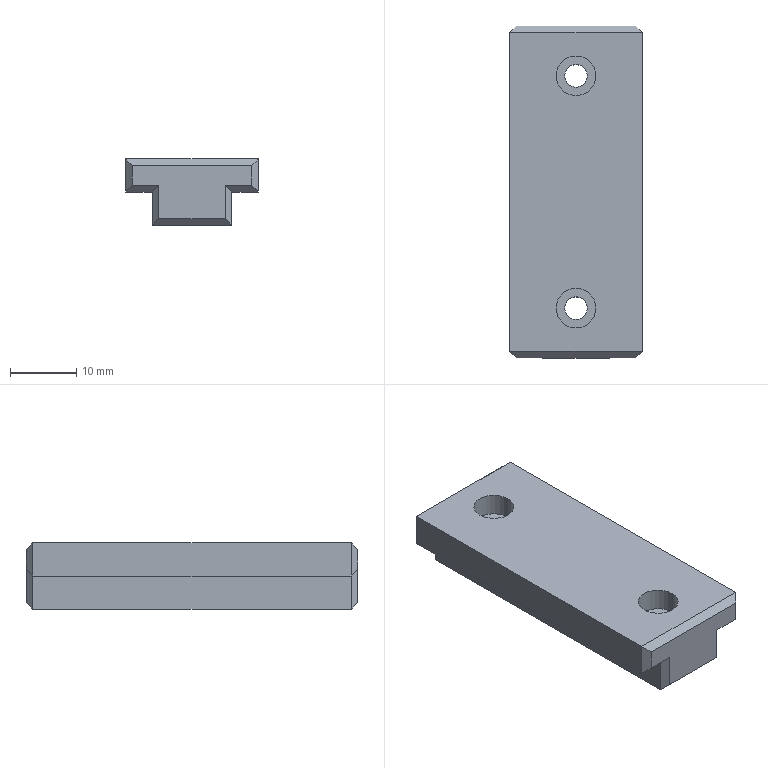Part | SolidWorks | features Chamfer 1, Extrusion 1, HoleWzd 1 | 1 solid | 36 faces | box 20 x 50 x 10 mm | volume 7631 mm3 | plane 28 | cylinder 8 | commonest cylinder face diameters 3.4 x4 6 x4
STEP:
#1=CARTESIAN_POINT('',(-3.,42.5,-3.4));
#2=VERTEX_POINT('',#1);
#3=CARTESIAN_POINT('',(3.,42.5,-3.4));
#4=VERTEX_POINT('',#3);
#5=CARTESIAN_POINT('',(0.,42.5,-3.4));
#6=DIRECTION('',(0.,0.,1.));
#7=DIRECTION('',(1.,0.,0.));
#8=AXIS2_PLACEMENT_3D('',#5,#6,#7);
#9=CIRCLE('',#8,3.);
#10=EDGE_CURVE('',#2,#4,#9,.T.);
#11=ORIENTED_EDGE('',*,*,#10,.F.);
#12=CARTESIAN_POINT('',(-3.,42.5,0.));
#13=VERTEX_POINT('',#12);
#14=CARTESIAN_POINT('',(-3.,42.5,0.));
#15=DIRECTION('',(0.,0.,1.));
#16=VECTOR('',#15,1000.);
#17=LINE('',#14,#16);
#18=EDGE_CURVE('',#2,#13,#17,.T.);
#19=ORIENTED_EDGE('',*,*,#18,.T.);
#20=CARTESIAN_POINT('',(3.,42.5,0.));
#21=VERTEX_POINT('',#20);
#22=CARTESIAN_POINT('',(0.,42.5,0.));
#23=DIRECTION('',(0.,0.,1.));
#24=DIRECTION('',(1.,0.,0.));
#25=AXIS2_PLACEMENT_3D('',#22,#23,#24);
#26=CIRCLE('',#25,3.);
#27=EDGE_CURVE('',#13,#21,#26,.T.);
#28=ORIENTED_EDGE('',*,*,#27,.T.);
#29=CARTESIAN_POINT('',(3.,42.5,0.));
#30=DIRECTION('',(0.,0.,1.));
#31=VECTOR('',#30,1000.);
#32=LINE('',#29,#31);
#33=EDGE_CURVE('',#4,#21,#32,.T.);
#34=ORIENTED_EDGE('',*,*,#33,.F.);
#35=EDGE_LOOP('',(#11,#19,#28,#34));
#36=FACE_OUTER_BOUND('',#35,.T.);
#37=CARTESIAN_POINT('',(0.,42.5,0.));
#38=DIRECTION('',(0.,0.,1.));
#39=DIRECTION('',(1.,0.,0.));
#40=AXIS2_PLACEMENT_3D('',#37,#38,#39);
#41=CYLINDRICAL_SURFACE('',#40,3.);
#42=ADVANCED_FACE('',(#36),#41,.F.);
#43=CARTESIAN_POINT('',(-1.7,42.5,-10.));
#44=VERTEX_POINT('',#43);
#45=CARTESIAN_POINT('',(1.7,42.5,-10.));
#46=VERTEX_POINT('',#45);
#47=CARTESIAN_POINT('',(0.,42.5,-10.));
#48=DIRECTION('',(0.,0.,1.));
#49=DIRECTION('',(1.,0.,0.));
#50=AXIS2_PLACEMENT_3D('',#47,#48,#49);
#51=CIRCLE('',#50,1.7);
#52=EDGE_CURVE('',#44,#46,#51,.T.);
#53=ORIENTED_EDGE('',*,*,#52,.F.);
#54=CARTESIAN_POINT('',(-1.7,42.5,-3.4));
#55=VERTEX_POINT('',#54);
#56=CARTESIAN_POINT('',(-1.7,42.5,0.));
#57=DIRECTION('',(0.,0.,1.));
#58=VECTOR('',#57,1000.);
#59=LINE('',#56,#58);
#60=EDGE_CURVE('',#44,#55,#59,.T.);
#61=ORIENTED_EDGE('',*,*,#60,.T.);
#62=CARTESIAN_POINT('',(1.7,42.5,-3.4));
#63=VERTEX_POINT('',#62);
#64=CARTESIAN_POINT('',(0.,42.5,-3.4));
#65=DIRECTION('',(0.,0.,1.));
#66=DIRECTION('',(1.,0.,0.));
#67=AXIS2_PLACEMENT_3D('',#64,#65,#66);
#68=CIRCLE('',#67,1.7);
#69=EDGE_CURVE('',#55,#63,#68,.T.);
#70=ORIENTED_EDGE('',*,*,#69,.T.);
#71=CARTESIAN_POINT('',(1.7,42.5,0.));
#72=DIRECTION('',(0.,0.,1.));
#73=VECTOR('',#72,1000.);
#74=LINE('',#71,#73);
#75=EDGE_CURVE('',#46,#63,#74,.T.);
#76=ORIENTED_EDGE('',*,*,#75,.F.);
#77=EDGE_LOOP('',(#53,#61,#70,#76));
#78=FACE_OUTER_BOUND('',#77,.T.);
#79=CARTESIAN_POINT('',(0.,42.5,0.));
#80=DIRECTION('',(0.,0.,1.));
#81=DIRECTION('',(1.,0.,0.));
#82=AXIS2_PLACEMENT_3D('',#79,#80,#81);
#83=CYLINDRICAL_SURFACE('',#82,1.7);
#84=ADVANCED_FACE('',(#78),#83,.F.);
#85=CARTESIAN_POINT('',(-3.,7.5,-3.4));
#86=VERTEX_POINT('',#85);
#87=CARTESIAN_POINT('',(3.,7.5,-3.4));
#88=VERTEX_POINT('',#87);
#89=CARTESIAN_POINT('',(0.,7.5,-3.4));
#90=DIRECTION('',(0.,0.,1.));
#91=DIRECTION('',(1.,0.,0.));
#92=AXIS2_PLACEMENT_3D('',#89,#90,#91);
#93=CIRCLE('',#92,3.);
#94=EDGE_CURVE('',#86,#88,#93,.T.);
#95=ORIENTED_EDGE('',*,*,#94,.F.);
#96=CARTESIAN_POINT('',(-3.,7.5,0.));
#97=VERTEX_POINT('',#96);
#98=CARTESIAN_POINT('',(-3.,7.5,0.));
#99=DIRECTION('',(0.,0.,1.));
#100=VECTOR('',#99,1000.);
#101=LINE('',#98,#100);
#102=EDGE_CURVE('',#86,#97,#101,.T.);
#103=ORIENTED_EDGE('',*,*,#102,.T.);
#104=CARTESIAN_POINT('',(3.,7.5,0.));
#105=VERTEX_POINT('',#104);
#106=CARTESIAN_POINT('',(0.,7.5,0.));
#107=DIRECTION('',(0.,0.,1.));
#108=DIRECTION('',(1.,0.,0.));
#109=AXIS2_PLACEMENT_3D('',#106,#107,#108);
#110=CIRCLE('',#109,3.);
#111=EDGE_CURVE('',#97,#105,#110,.T.);
#112=ORIENTED_EDGE('',*,*,#111,.T.);
#113=CARTESIAN_POINT('',(3.,7.5,0.));
#114=DIRECTION('',(0.,0.,1.));
#115=VECTOR('',#114,1000.);
#116=LINE('',#113,#115);
#117=EDGE_CURVE('',#88,#105,#116,.T.);
#118=ORIENTED_EDGE('',*,*,#117,.F.);
#119=EDGE_LOOP('',(#95,#103,#112,#118));
#120=FACE_OUTER_BOUND('',#119,.T.);
#121=CARTESIAN_POINT('',(0.,7.5,0.));
#122=DIRECTION('',(0.,0.,1.));
#123=DIRECTION('',(1.,0.,0.));
#124=AXIS2_PLACEMENT_3D('',#121,#122,#123);
#125=CYLINDRICAL_SURFACE('',#124,3.);
#126=ADVANCED_FACE('',(#120),#125,.F.);
#127=CARTESIAN_POINT('',(-1.7,7.5,-10.));
#128=VERTEX_POINT('',#127);
#129=CARTESIAN_POINT('',(1.7,7.5,-10.));
#130=VERTEX_POINT('',#129);
#131=CARTESIAN_POINT('',(0.,7.5,-10.));
#132=DIRECTION('',(0.,0.,1.));
#133=DIRECTION('',(1.,0.,0.));
#134=AXIS2_PLACEMENT_3D('',#131,#132,#133);
#135=CIRCLE('',#134,1.7);
#136=EDGE_CURVE('',#128,#130,#135,.T.);
#137=ORIENTED_EDGE('',*,*,#136,.F.);
#138=CARTESIAN_POINT('',(-1.7,7.5,-3.4));
#139=VERTEX_POINT('',#138);
#140=CARTESIAN_POINT('',(-1.7,7.5,0.));
#141=DIRECTION('',(0.,0.,1.));
#142=VECTOR('',#141,1000.);
#143=LINE('',#140,#142);
#144=EDGE_CURVE('',#128,#139,#143,.T.);
#145=ORIENTED_EDGE('',*,*,#144,.T.);
#146=CARTESIAN_POINT('',(1.7,7.5,-3.4));
#147=VERTEX_POINT('',#146);
#148=CARTESIAN_POINT('',(0.,7.5,-3.4));
#149=DIRECTION('',(0.,0.,1.));
#150=DIRECTION('',(1.,0.,0.));
#151=AXIS2_PLACEMENT_3D('',#148,#149,#150);
#152=CIRCLE('',#151,1.7);
#153=EDGE_CURVE('',#139,#147,#152,.T.);
#154=ORIENTED_EDGE('',*,*,#153,.T.);
#155=CARTESIAN_POINT('',(1.7,7.5,0.));
#156=DIRECTION('',(0.,0.,1.));
#157=VECTOR('',#156,1000.);
#158=LINE('',#155,#157);
#159=EDGE_CURVE('',#130,#147,#158,.T.);
#160=ORIENTED_EDGE('',*,*,#159,.F.);
#161=EDGE_LOOP('',(#137,#145,#154,#160));
#162=FACE_OUTER_BOUND('',#161,.T.);
#163=CARTESIAN_POINT('',(0.,7.5,0.));
#164=DIRECTION('',(0.,0.,1.));
#165=DIRECTION('',(1.,0.,0.));
#166=AXIS2_PLACEMENT_3D('',#163,#164,#165);
#167=CYLINDRICAL_SURFACE('',#166,1.7);
#168=ADVANCED_FACE('',(#162),#167,.F.);
#169=CARTESIAN_POINT('',(0.,7.5,0.));
#170=DIRECTION('',(0.,0.,1.));
#171=DIRECTION('',(1.,0.,0.));
#172=AXIS2_PLACEMENT_3D('',#169,#170,#171);
#173=CIRCLE('',#172,3.);
#174=EDGE_CURVE('',#105,#97,#173,.T.);
#175=ORIENTED_EDGE('',*,*,#174,.F.);
#176=ORIENTED_EDGE('',*,*,#111,.F.);
#177=EDGE_LOOP('',(#175,#176));
#178=FACE_BOUND('',#177,.T.);
#179=CARTESIAN_POINT('',(10.,49.,0.));
#180=VERTEX_POINT('',#179);
#181=CARTESIAN_POINT('',(10.,1.,0.));
#182=VERTEX_POINT('',#181);
#183=CARTESIAN_POINT('',(10.,50.,0.));
#184=DIRECTION('',(0.,-1.,0.));
#185=VECTOR('',#184,1000.);
#186=LINE('',#183,#185);
#187=EDGE_CURVE('',#180,#182,#186,.T.);
#188=ORIENTED_EDGE('',*,*,#187,.F.);
#189=CARTESIAN_POINT('',(-10.,49.,0.));
#190=VERTEX_POINT('',#189);
#191=CARTESIAN_POINT('',(10.,49.,0.));
#192=DIRECTION('',(-1.,0.,0.));
#193=VECTOR('',#192,1000.);
#194=LINE('',#191,#193);
#195=EDGE_CURVE('',#180,#190,#194,.T.);
#196=ORIENTED_EDGE('',*,*,#195,.T.);
#197=CARTESIAN_POINT('',(-10.,1.,0.));
#198=VERTEX_POINT('',#197);
#199=CARTESIAN_POINT('',(-10.,50.,0.));
#200=DIRECTION('',(0.,-1.,0.));
#201=VECTOR('',#200,1000.);
#202=LINE('',#199,#201);
#203=EDGE_CURVE('',#190,#198,#202,.T.);
#204=ORIENTED_EDGE('',*,*,#203,.T.);
#205=CARTESIAN_POINT('',(10.,1.,0.));
#206=DIRECTION('',(1.,0.,0.));
#207=VECTOR('',#206,1000.);
#208=LINE('',#205,#207);
#209=EDGE_CURVE('',#198,#182,#208,.T.);
#210=ORIENTED_EDGE('',*,*,#209,.T.);
#211=EDGE_LOOP('',(#188,#196,#204,#210));
#212=FACE_OUTER_BOUND('',#211,.T.);
#213=CARTESIAN_POINT('',(0.,42.5,0.));
#214=DIRECTION('',(0.,0.,1.));
#215=DIRECTION('',(1.,0.,0.));
#216=AXIS2_PLACEMENT_3D('',#213,#214,#215);
#217=CIRCLE('',#216,3.);
#218=EDGE_CURVE('',#21,#13,#217,.T.);
#219=ORIENTED_EDGE('',*,*,#218,.F.);
#220=ORIENTED_EDGE('',*,*,#27,.F.);
#221=EDGE_LOOP('',(#219,#220));
#222=FACE_BOUND('',#221,.T.);
#223=CARTESIAN_POINT('',(10.,50.,0.));
#224=DIRECTION('',(0.,0.,-1.));
#225=DIRECTION('',(-1.,0.,0.));
#226=AXIS2_PLACEMENT_3D('',#223,#224,#225);
#227=PLANE('',#226);
#228=ADVANCED_FACE('',(#178,#212,#222),#227,.F.);
#229=ORIENTED_EDGE('',*,*,#203,.F.);
#230=CARTESIAN_POINT('',(-10.,49.,-5.));
#231=VERTEX_POINT('',#230);
#232=CARTESIAN_POINT('',(-10.,49.,0.));
#233=DIRECTION('',(0.,0.,-1.));
#234=VECTOR('',#233,1000.);
#235=LINE('',#232,#234);
#236=EDGE_CURVE('',#190,#231,#235,.T.);
#237=ORIENTED_EDGE('',*,*,#236,.T.);
#238=CARTESIAN_POINT('',(-10.,1.,-5.));
#239=VERTEX_POINT('',#238);
#240=CARTESIAN_POINT('',(-10.,50.,-5.));
#241=DIRECTION('',(0.,-1.,0.));
#242=VECTOR('',#241,1000.);
#243=LINE('',#240,#242);
#244=EDGE_CURVE('',#231,#239,#243,.T.);
#245=ORIENTED_EDGE('',*,*,#244,.T.);
#246=CARTESIAN_POINT('',(-10.,1.,0.));
#247=DIRECTION('',(0.,0.,1.));
#248=VECTOR('',#247,1000.);
#249=LINE('',#246,#248);
#250=EDGE_CURVE('',#239,#198,#249,.T.);
#251=ORIENTED_EDGE('',*,*,#250,.T.);
#252=EDGE_LOOP('',(#229,#237,#245,#251));
#253=FACE_OUTER_BOUND('',#252,.T.);
#254=CARTESIAN_POINT('',(-10.,50.,0.));
#255=DIRECTION('',(1.,0.,0.));
#256=DIRECTION('',(0.,0.,-1.));
#257=AXIS2_PLACEMENT_3D('',#254,#255,#256);
#258=PLANE('',#257);
#259=ADVANCED_FACE('',(#253),#258,.F.);
#260=CARTESIAN_POINT('',(10.,49.,-5.));
#261=VERTEX_POINT('',#260);
#262=CARTESIAN_POINT('',(10.,1.,-5.));
#263=VERTEX_POINT('',#262);
#264=CARTESIAN_POINT('',(10.,50.,-5.));
#265=DIRECTION('',(0.,-1.,0.));
#266=VECTOR('',#265,1000.);
#267=LINE('',#264,#266);
#268=EDGE_CURVE('',#261,#263,#267,.T.);
#269=ORIENTED_EDGE('',*,*,#268,.F.);
#270=CARTESIAN_POINT('',(10.,49.,0.));
#271=DIRECTION('',(0.,0.,1.));
#272=VECTOR('',#271,1000.);
#273=LINE('',#270,#272);
#274=EDGE_CURVE('',#261,#180,#273,.T.);
#275=ORIENTED_EDGE('',*,*,#274,.T.);
#276=ORIENTED_EDGE('',*,*,#187,.T.);
#277=CARTESIAN_POINT('',(10.,1.,-5.));
#278=DIRECTION('',(0.,0.,-1.));
#279=VECTOR('',#278,1000.);
#280=LINE('',#277,#279);
#281=EDGE_CURVE('',#182,#263,#280,.T.);
#282=ORIENTED_EDGE('',*,*,#281,.T.);
#283=EDGE_LOOP('',(#269,#275,#276,#282));
#284=FACE_OUTER_BOUND('',#283,.T.);
#285=CARTESIAN_POINT('',(10.,50.,0.));
#286=DIRECTION('',(-1.,0.,0.));
#287=DIRECTION('',(0.,0.,1.));
#288=AXIS2_PLACEMENT_3D('',#285,#286,#287);
#289=PLANE('',#288);
#290=ADVANCED_FACE('',(#284),#289,.F.);
#291=CARTESIAN_POINT('',(6.,49.,-5.));
#292=VERTEX_POINT('',#291);
#293=CARTESIAN_POINT('',(6.,1.,-5.));
#294=VERTEX_POINT('',#293);
#295=CARTESIAN_POINT('',(6.,50.,-5.));
#296=DIRECTION('',(0.,-1.,0.));
#297=VECTOR('',#296,1000.);
#298=LINE('',#295,#297);
#299=EDGE_CURVE('',#292,#294,#298,.T.);
#300=ORIENTED_EDGE('',*,*,#299,.F.);
#301=CARTESIAN_POINT('',(10.,49.,-5.));
#302=DIRECTION('',(1.,0.,0.));
#303=VECTOR('',#302,1000.);
#304=LINE('',#301,#303);
#305=EDGE_CURVE('',#292,#261,#304,.T.);
#306=ORIENTED_EDGE('',*,*,#305,.T.);
#307=ORIENTED_EDGE('',*,*,#268,.T.);
#308=CARTESIAN_POINT('',(6.,1.,-5.));
#309=DIRECTION('',(-1.,0.,0.));
#310=VECTOR('',#309,1000.);
#311=LINE('',#308,#310);
#312=EDGE_CURVE('',#263,#294,#311,.T.);
#313=ORIENTED_EDGE('',*,*,#312,.T.);
#314=EDGE_LOOP('',(#300,#306,#307,#313));
#315=FACE_OUTER_BOUND('',#314,.T.);
#316=CARTESIAN_POINT('',(10.,50.,-5.));
#317=DIRECTION('',(0.,0.,1.));
#318=DIRECTION('',(1.,0.,0.));
#319=AXIS2_PLACEMENT_3D('',#316,#317,#318);
#320=PLANE('',#319);
#321=ADVANCED_FACE('',(#315),#320,.F.);
#322=CARTESIAN_POINT('',(6.,49.,-10.));
#323=VERTEX_POINT('',#322);
#324=CARTESIAN_POINT('',(6.,1.,-10.));
#325=VERTEX_POINT('',#324);
#326=CARTESIAN_POINT('',(6.,50.,-10.));
#327=DIRECTION('',(0.,-1.,0.));
#328=VECTOR('',#327,1000.);
#329=LINE('',#326,#328);
#330=EDGE_CURVE('',#323,#325,#329,.T.);
#331=ORIENTED_EDGE('',*,*,#330,.F.);
#332=CARTESIAN_POINT('',(6.,49.,-5.));
#333=DIRECTION('',(0.,0.,1.));
#334=VECTOR('',#333,1000.);
#335=LINE('',#332,#334);
#336=EDGE_CURVE('',#323,#292,#335,.T.);
#337=ORIENTED_EDGE('',*,*,#336,.T.);
#338=ORIENTED_EDGE('',*,*,#299,.T.);
#339=CARTESIAN_POINT('',(6.,1.,-10.));
#340=DIRECTION('',(0.,0.,-1.));
#341=VECTOR('',#340,1000.);
#342=LINE('',#339,#341);
#343=EDGE_CURVE('',#294,#325,#342,.T.);
#344=ORIENTED_EDGE('',*,*,#343,.T.);
#345=EDGE_LOOP('',(#331,#337,#338,#344));
#346=FACE_OUTER_BOUND('',#345,.T.);
#347=CARTESIAN_POINT('',(6.,50.,-5.));
#348=DIRECTION('',(-1.,0.,0.));
#349=DIRECTION('',(0.,0.,1.));
#350=AXIS2_PLACEMENT_3D('',#347,#348,#349);
#351=PLANE('',#350);
#352=ADVANCED_FACE('',(#346),#351,.F.);
#353=CARTESIAN_POINT('',(0.,42.5,-10.));
#354=DIRECTION('',(0.,0.,1.));
#355=DIRECTION('',(1.,0.,0.));
#356=AXIS2_PLACEMENT_3D('',#353,#354,#355);
#357=CIRCLE('',#356,1.7);
#358=EDGE_CURVE('',#46,#44,#357,.T.);
#359=ORIENTED_EDGE('',*,*,#358,.T.);
#360=ORIENTED_EDGE('',*,*,#52,.T.);
#361=EDGE_LOOP('',(#359,#360));
#362=FACE_BOUND('',#361,.T.);
#363=CARTESIAN_POINT('',(0.,7.5,-10.));
#364=DIRECTION('',(0.,0.,1.));
#365=DIRECTION('',(1.,0.,0.));
#366=AXIS2_PLACEMENT_3D('',#363,#364,#365);
#367=CIRCLE('',#366,1.7);
#368=EDGE_CURVE('',#130,#128,#367,.T.);
#369=ORIENTED_EDGE('',*,*,#368,.T.);
#370=ORIENTED_EDGE('',*,*,#136,.T.);
#371=EDGE_LOOP('',(#369,#370));
#372=FACE_BOUND('',#371,.T.);
#373=CARTESIAN_POINT('',(-6.,49.,-10.));
#374=VERTEX_POINT('',#373);
#375=CARTESIAN_POINT('',(-6.,1.,-10.));
#376=VERTEX_POINT('',#375);
#377=CARTESIAN_POINT('',(-6.,50.,-10.));
#378=DIRECTION('',(0.,-1.,0.));
#379=VECTOR('',#378,1000.);
#380=LINE('',#377,#379);
#381=EDGE_CURVE('',#374,#376,#380,.T.);
#382=ORIENTED_EDGE('',*,*,#381,.F.);
#383=CARTESIAN_POINT('',(-6.,49.,-10.));
#384=DIRECTION('',(1.,0.,0.));
#385=VECTOR('',#384,1000.);
#386=LINE('',#383,#385);
#387=EDGE_CURVE('',#374,#323,#386,.T.);
#388=ORIENTED_EDGE('',*,*,#387,.T.);
#389=ORIENTED_EDGE('',*,*,#330,.T.);
#390=CARTESIAN_POINT('',(-6.,1.,-10.));
#391=DIRECTION('',(-1.,0.,0.));
#392=VECTOR('',#391,1000.);
#393=LINE('',#390,#392);
#394=EDGE_CURVE('',#325,#376,#393,.T.);
#395=ORIENTED_EDGE('',*,*,#394,.T.);
#396=EDGE_LOOP('',(#382,#388,#389,#395));
#397=FACE_OUTER_BOUND('',#396,.T.);
#398=CARTESIAN_POINT('',(-6.,50.,-10.));
#399=DIRECTION('',(0.,0.,1.));
#400=DIRECTION('',(1.,0.,0.));
#401=AXIS2_PLACEMENT_3D('',#398,#399,#400);
#402=PLANE('',#401);
#403=ADVANCED_FACE('',(#362,#372,#397),#402,.F.);
#404=CARTESIAN_POINT('',(-6.,49.,-5.));
#405=VERTEX_POINT('',#404);
#406=CARTESIAN_POINT('',(-6.,1.,-5.));
#407=VERTEX_POINT('',#406);
#408=CARTESIAN_POINT('',(-6.,50.,-5.));
#409=DIRECTION('',(0.,-1.,0.));
#410=VECTOR('',#409,1000.);
#411=LINE('',#408,#410);
#412=EDGE_CURVE('',#405,#407,#411,.T.);
#413=ORIENTED_EDGE('',*,*,#412,.F.);
#414=CARTESIAN_POINT('',(-6.,49.,-5.));
#415=DIRECTION('',(0.,0.,-1.));
#416=VECTOR('',#415,1000.);
#417=LINE('',#414,#416);
#418=EDGE_CURVE('',#405,#374,#417,.T.);
#419=ORIENTED_EDGE('',*,*,#418,.T.);
#420=ORIENTED_EDGE('',*,*,#381,.T.);
#421=CARTESIAN_POINT('',(-6.,1.,-5.));
#422=DIRECTION('',(0.,0.,1.));
#423=VECTOR('',#422,1000.);
#424=LINE('',#421,#423);
#425=EDGE_CURVE('',#376,#407,#424,.T.);
#426=ORIENTED_EDGE('',*,*,#425,.T.);
#427=EDGE_LOOP('',(#413,#419,#420,#426));
#428=FACE_OUTER_BOUND('',#427,.T.);
#429=CARTESIAN_POINT('',(-6.,50.,-5.));
#430=DIRECTION('',(1.,0.,0.));
#431=DIRECTION('',(0.,0.,-1.));
#432=AXIS2_PLACEMENT_3D('',#429,#430,#431);
#433=PLANE('',#432);
#434=ADVANCED_FACE('',(#428),#433,.F.);
#435=ORIENTED_EDGE('',*,*,#244,.F.);
#436=CARTESIAN_POINT('',(-10.,49.,-5.));
#437=DIRECTION('',(1.,0.,0.));
#438=VECTOR('',#437,1000.);
#439=LINE('',#436,#438);
#440=EDGE_CURVE('',#231,#405,#439,.T.);
#441=ORIENTED_EDGE('',*,*,#440,.T.);
#442=ORIENTED_EDGE('',*,*,#412,.T.);
#443=CARTESIAN_POINT('',(-10.,1.,-5.));
#444=DIRECTION('',(-1.,0.,0.));
#445=VECTOR('',#444,1000.);
#446=LINE('',#443,#445);
#447=EDGE_CURVE('',#407,#239,#446,.T.);
#448=ORIENTED_EDGE('',*,*,#447,.T.);
#449=EDGE_LOOP('',(#435,#441,#442,#448));
#450=FACE_OUTER_BOUND('',#449,.T.);
#451=CARTESIAN_POINT('',(-10.,50.,-5.));
#452=DIRECTION('',(0.,0.,1.));
#453=DIRECTION('',(1.,0.,0.));
#454=AXIS2_PLACEMENT_3D('',#451,#452,#453);
#455=PLANE('',#454);
#456=ADVANCED_FACE('',(#450),#455,.F.);
#457=CARTESIAN_POINT('',(-9.,50.,-4.));
#458=VERTEX_POINT('',#457);
#459=CARTESIAN_POINT('',(-9.,50.,-1.));
#460=VERTEX_POINT('',#459);
#461=CARTESIAN_POINT('',(-9.,50.,0.));
#462=DIRECTION('',(0.,0.,1.));
#463=VECTOR('',#462,1000.);
#464=LINE('',#461,#463);
#465=EDGE_CURVE('',#458,#460,#464,.T.);
#466=ORIENTED_EDGE('',*,*,#465,.T.);
#467=CARTESIAN_POINT('',(9.,50.,-1.));
#468=VERTEX_POINT('',#467);
#469=CARTESIAN_POINT('',(0.,50.,-1.));
#470=DIRECTION('',(1.,0.,0.));
#471=VECTOR('',#470,1000.);
#472=LINE('',#469,#471);
#473=EDGE_CURVE('',#460,#468,#472,.T.);
#474=ORIENTED_EDGE('',*,*,#473,.T.);
#475=CARTESIAN_POINT('',(9.,50.,-4.));
#476=VERTEX_POINT('',#475);
#477=CARTESIAN_POINT('',(9.,50.,0.));
#478=DIRECTION('',(0.,0.,-1.));
#479=VECTOR('',#478,1000.);
#480=LINE('',#477,#479);
#481=EDGE_CURVE('',#468,#476,#480,.T.);
#482=ORIENTED_EDGE('',*,*,#481,.T.);
#483=CARTESIAN_POINT('',(5.,50.,-4.));
#484=VERTEX_POINT('',#483);
#485=CARTESIAN_POINT('',(0.,50.,-4.));
#486=DIRECTION('',(-1.,0.,0.));
#487=VECTOR('',#486,1000.);
#488=LINE('',#485,#487);
#489=EDGE_CURVE('',#476,#484,#488,.T.);
#490=ORIENTED_EDGE('',*,*,#489,.T.);
#491=CARTESIAN_POINT('',(5.,50.,-9.));
#492=VERTEX_POINT('',#491);
#493=CARTESIAN_POINT('',(5.,50.,0.));
#494=DIRECTION('',(0.,0.,-1.));
#495=VECTOR('',#494,1000.);
#496=LINE('',#493,#495);
#497=EDGE_CURVE('',#484,#492,#496,.T.);
#498=ORIENTED_EDGE('',*,*,#497,.T.);
#499=CARTESIAN_POINT('',(-5.,50.,-9.));
#500=VERTEX_POINT('',#499);
#501=CARTESIAN_POINT('',(0.,50.,-9.));
#502=DIRECTION('',(-1.,0.,0.));
#503=VECTOR('',#502,1000.);
#504=LINE('',#501,#503);
#505=EDGE_CURVE('',#492,#500,#504,.T.);
#506=ORIENTED_EDGE('',*,*,#505,.T.);
#507=CARTESIAN_POINT('',(-5.,50.,-4.));
#508=VERTEX_POINT('',#507);
#509=CARTESIAN_POINT('',(-5.,50.,0.));
#510=DIRECTION('',(0.,0.,1.));
#511=VECTOR('',#510,1000.);
#512=LINE('',#509,#511);
#513=EDGE_CURVE('',#500,#508,#512,.T.);
#514=ORIENTED_EDGE('',*,*,#513,.T.);
#515=CARTESIAN_POINT('',(0.,50.,-4.));
#516=DIRECTION('',(-1.,0.,0.));
#517=VECTOR('',#516,1000.);
#518=LINE('',#515,#517);
#519=EDGE_CURVE('',#508,#458,#518,.T.);
#520=ORIENTED_EDGE('',*,*,#519,.T.);
#521=EDGE_LOOP('',(#466,#474,#482,#490,#498,#506,#514,#520));
#522=FACE_OUTER_BOUND('',#521,.T.);
#523=CARTESIAN_POINT('',(0.,50.,0.));
#524=DIRECTION('',(0.,-1.,0.));
#525=DIRECTION('',(0.,0.,-1.));
#526=AXIS2_PLACEMENT_3D('',#523,#524,#525);
#527=PLANE('',#526);
#528=ADVANCED_FACE('',(#522),#527,.F.);
#529=CARTESIAN_POINT('',(9.,0.,-4.));
#530=VERTEX_POINT('',#529);
#531=CARTESIAN_POINT('',(9.,0.,-1.));
#532=VERTEX_POINT('',#531);
#533=CARTESIAN_POINT('',(9.,0.,0.));
#534=DIRECTION('',(0.,0.,1.));
#535=VECTOR('',#534,1000.);
#536=LINE('',#533,#535);
#537=EDGE_CURVE('',#530,#532,#536,.T.);
#538=ORIENTED_EDGE('',*,*,#537,.T.);
#539=CARTESIAN_POINT('',(-9.,0.,-1.));
#540=VERTEX_POINT('',#539);
#541=CARTESIAN_POINT('',(-10.,0.,-1.));
#542=DIRECTION('',(-1.,0.,0.));
#543=VECTOR('',#542,1000.);
#544=LINE('',#541,#543);
#545=EDGE_CURVE('',#532,#540,#544,.T.);
#546=ORIENTED_EDGE('',*,*,#545,.T.);
#547=CARTESIAN_POINT('',(-9.,0.,-4.));
#548=VERTEX_POINT('',#547);
#549=CARTESIAN_POINT('',(-9.,0.,-5.));
#550=DIRECTION('',(0.,0.,-1.));
#551=VECTOR('',#550,1000.);
#552=LINE('',#549,#551);
#553=EDGE_CURVE('',#540,#548,#552,.T.);
#554=ORIENTED_EDGE('',*,*,#553,.T.);
#555=CARTESIAN_POINT('',(-5.,0.,-4.));
#556=VERTEX_POINT('',#555);
#557=CARTESIAN_POINT('',(-6.,0.,-4.));
#558=DIRECTION('',(1.,0.,0.));
#559=VECTOR('',#558,1000.);
#560=LINE('',#557,#559);
#561=EDGE_CURVE('',#548,#556,#560,.T.);
#562=ORIENTED_EDGE('',*,*,#561,.T.);
#563=CARTESIAN_POINT('',(-5.,0.,-9.));
#564=VERTEX_POINT('',#563);
#565=CARTESIAN_POINT('',(-5.,0.,-10.));
#566=DIRECTION('',(0.,0.,-1.));
#567=VECTOR('',#566,1000.);
#568=LINE('',#565,#567);
#569=EDGE_CURVE('',#556,#564,#568,.T.);
#570=ORIENTED_EDGE('',*,*,#569,.T.);
#571=CARTESIAN_POINT('',(5.,0.,-9.));
#572=VERTEX_POINT('',#571);
#573=CARTESIAN_POINT('',(6.,0.,-9.));
#574=DIRECTION('',(1.,0.,0.));
#575=VECTOR('',#574,1000.);
#576=LINE('',#573,#575);
#577=EDGE_CURVE('',#564,#572,#576,.T.);
#578=ORIENTED_EDGE('',*,*,#577,.T.);
#579=CARTESIAN_POINT('',(5.,0.,-4.));
#580=VERTEX_POINT('',#579);
#581=CARTESIAN_POINT('',(5.,0.,-5.));
#582=DIRECTION('',(0.,0.,1.));
#583=VECTOR('',#582,1000.);
#584=LINE('',#581,#583);
#585=EDGE_CURVE('',#572,#580,#584,.T.);
#586=ORIENTED_EDGE('',*,*,#585,.T.);
#587=CARTESIAN_POINT('',(10.,0.,-4.));
#588=DIRECTION('',(1.,0.,0.));
#589=VECTOR('',#588,1000.);
#590=LINE('',#587,#589);
#591=EDGE_CURVE('',#580,#530,#590,.T.);
#592=ORIENTED_EDGE('',*,*,#591,.T.);
#593=EDGE_LOOP('',(#538,#546,#554,#562,#570,#578,#586,#592));
#594=FACE_OUTER_BOUND('',#593,.T.);
#595=CARTESIAN_POINT('',(0.,0.,0.));
#596=DIRECTION('',(0.,-1.,0.));
#597=DIRECTION('',(0.,0.,-1.));
#598=AXIS2_PLACEMENT_3D('',#595,#596,#597);
#599=PLANE('',#598);
#600=ADVANCED_FACE('',(#594),#599,.T.);
#601=CARTESIAN_POINT('',(2.,53.,-6.));
#602=DIRECTION('',(-0.5774,0.5774,0.5774));
#603=VECTOR('',#602,1000.);
#604=LINE('',#601,#603);
#605=EDGE_CURVE('',#323,#492,#604,.T.);
#606=ORIENTED_EDGE('',*,*,#605,.F.);
#607=ORIENTED_EDGE('',*,*,#387,.F.);
#608=CARTESIAN_POINT('',(-3.333,51.667,-7.333));
#609=DIRECTION('',(-0.5774,-0.5774,-0.5774));
#610=VECTOR('',#609,1000.);
#611=LINE('',#608,#610);
#612=EDGE_CURVE('',#500,#374,#611,.T.);
#613=ORIENTED_EDGE('',*,*,#612,.F.);
#614=ORIENTED_EDGE('',*,*,#505,.F.);
#615=EDGE_LOOP('',(#606,#607,#613,#614));
#616=FACE_OUTER_BOUND('',#615,.T.);
#617=CARTESIAN_POINT('',(0.,50.,-9.));
#618=DIRECTION('',(0.,-0.7071,0.7071));
#619=DIRECTION('',(-1.,0.,0.));
#620=AXIS2_PLACEMENT_3D('',#617,#618,#619);
#621=PLANE('',#620);
#622=ADVANCED_FACE('',(#616),#621,.F.);
#623=ORIENTED_EDGE('',*,*,#612,.T.);
#624=ORIENTED_EDGE('',*,*,#418,.F.);
#625=CARTESIAN_POINT('',(-3.333,51.667,-2.333));
#626=DIRECTION('',(-0.5774,-0.5774,-0.5774));
#627=VECTOR('',#626,1000.);
#628=LINE('',#625,#627);
#629=EDGE_CURVE('',#508,#405,#628,.T.);
#630=ORIENTED_EDGE('',*,*,#629,.F.);
#631=ORIENTED_EDGE('',*,*,#513,.F.);
#632=EDGE_LOOP('',(#623,#624,#630,#631));
#633=FACE_OUTER_BOUND('',#632,.T.);
#634=CARTESIAN_POINT('',(-5.,50.,0.));
#635=DIRECTION('',(0.7071,-0.7071,0.));
#636=DIRECTION('',(0.,0.,1.));
#637=AXIS2_PLACEMENT_3D('',#634,#635,#636);
#638=PLANE('',#637);
#639=ADVANCED_FACE('',(#633),#638,.F.);
#640=ORIENTED_EDGE('',*,*,#605,.T.);
#641=ORIENTED_EDGE('',*,*,#497,.F.);
#642=CARTESIAN_POINT('',(3.667,51.333,-2.667));
#643=DIRECTION('',(-0.5774,0.5774,0.5774));
#644=VECTOR('',#643,1000.);
#645=LINE('',#642,#644);
#646=EDGE_CURVE('',#292,#484,#645,.T.);
#647=ORIENTED_EDGE('',*,*,#646,.F.);
#648=ORIENTED_EDGE('',*,*,#336,.F.);
#649=EDGE_LOOP('',(#640,#641,#647,#648));
#650=FACE_OUTER_BOUND('',#649,.T.);
#651=CARTESIAN_POINT('',(5.,50.,0.));
#652=DIRECTION('',(-0.7071,-0.7071,0.));
#653=DIRECTION('',(0.,0.,-1.));
#654=AXIS2_PLACEMENT_3D('',#651,#652,#653);
#655=PLANE('',#654);
#656=ADVANCED_FACE('',(#650),#655,.F.);
#657=ORIENTED_EDGE('',*,*,#629,.T.);
#658=ORIENTED_EDGE('',*,*,#440,.F.);
#659=CARTESIAN_POINT('',(-6.,53.,-1.));
#660=DIRECTION('',(-0.5774,-0.5774,-0.5774));
#661=VECTOR('',#660,1000.);
#662=LINE('',#659,#661);
#663=EDGE_CURVE('',#458,#231,#662,.T.);
#664=ORIENTED_EDGE('',*,*,#663,.F.);
#665=ORIENTED_EDGE('',*,*,#519,.F.);
#666=EDGE_LOOP('',(#657,#658,#664,#665));
#667=FACE_OUTER_BOUND('',#666,.T.);
#668=CARTESIAN_POINT('',(0.,50.,-4.));
#669=DIRECTION('',(0.,-0.7071,0.7071));
#670=DIRECTION('',(-1.,0.,0.));
#671=AXIS2_PLACEMENT_3D('',#668,#669,#670);
#672=PLANE('',#671);
#673=ADVANCED_FACE('',(#667),#672,.F.);
#674=ORIENTED_EDGE('',*,*,#646,.T.);
#675=ORIENTED_EDGE('',*,*,#489,.F.);
#676=CARTESIAN_POINT('',(7.667,51.333,-2.667));
#677=DIRECTION('',(-0.5774,0.5774,0.5774));
#678=VECTOR('',#677,1000.);
#679=LINE('',#676,#678);
#680=EDGE_CURVE('',#261,#476,#679,.T.);
#681=ORIENTED_EDGE('',*,*,#680,.F.);
#682=ORIENTED_EDGE('',*,*,#305,.F.);
#683=EDGE_LOOP('',(#674,#675,#681,#682));
#684=FACE_OUTER_BOUND('',#683,.T.);
#685=CARTESIAN_POINT('',(0.,50.,-4.));
#686=DIRECTION('',(0.,-0.7071,0.7071));
#687=DIRECTION('',(-1.,0.,0.));
#688=AXIS2_PLACEMENT_3D('',#685,#686,#687);
#689=PLANE('',#688);
#690=ADVANCED_FACE('',(#684),#689,.F.);
#691=ORIENTED_EDGE('',*,*,#663,.T.);
#692=ORIENTED_EDGE('',*,*,#236,.F.);
#693=CARTESIAN_POINT('',(-9.333,49.667,-0.6667));
#694=DIRECTION('',(-0.5774,-0.5774,0.5774));
#695=VECTOR('',#694,1000.);
#696=LINE('',#693,#695);
#697=EDGE_CURVE('',#460,#190,#696,.T.);
#698=ORIENTED_EDGE('',*,*,#697,.F.);
#699=ORIENTED_EDGE('',*,*,#465,.F.);
#700=EDGE_LOOP('',(#691,#692,#698,#699));
#701=FACE_OUTER_BOUND('',#700,.T.);
#702=CARTESIAN_POINT('',(-9.,50.,0.));
#703=DIRECTION('',(0.7071,-0.7071,0.));
#704=DIRECTION('',(0.,0.,1.));
#705=AXIS2_PLACEMENT_3D('',#702,#703,#704);
#706=PLANE('',#705);
#707=ADVANCED_FACE('',(#701),#706,.F.);
#708=ORIENTED_EDGE('',*,*,#680,.T.);
#709=ORIENTED_EDGE('',*,*,#481,.F.);
#710=CARTESIAN_POINT('',(9.333,49.667,-0.6667));
#711=DIRECTION('',(-0.5774,0.5774,-0.5774));
#712=VECTOR('',#711,1000.);
#713=LINE('',#710,#712);
#714=EDGE_CURVE('',#180,#468,#713,.T.);
#715=ORIENTED_EDGE('',*,*,#714,.F.);
#716=ORIENTED_EDGE('',*,*,#274,.F.);
#717=EDGE_LOOP('',(#708,#709,#715,#716));
#718=FACE_OUTER_BOUND('',#717,.T.);
#719=CARTESIAN_POINT('',(9.,50.,0.));
#720=DIRECTION('',(-0.7071,-0.7071,0.));
#721=DIRECTION('',(0.,0.,-1.));
#722=AXIS2_PLACEMENT_3D('',#719,#720,#721);
#723=PLANE('',#722);
#724=ADVANCED_FACE('',(#718),#723,.F.);
#725=ORIENTED_EDGE('',*,*,#697,.T.);
#726=ORIENTED_EDGE('',*,*,#195,.F.);
#727=ORIENTED_EDGE('',*,*,#714,.T.);
#728=ORIENTED_EDGE('',*,*,#473,.F.);
#729=EDGE_LOOP('',(#725,#726,#727,#728));
#730=FACE_OUTER_BOUND('',#729,.T.);
#731=CARTESIAN_POINT('',(0.,50.,-1.));
#732=DIRECTION('',(0.,-0.7071,-0.7071));
#733=DIRECTION('',(1.,0.,0.));
#734=AXIS2_PLACEMENT_3D('',#731,#732,#733);
#735=PLANE('',#734);
#736=ADVANCED_FACE('',(#730),#735,.F.);
#737=CARTESIAN_POINT('',(2.,-3.,-6.));
#738=DIRECTION('',(0.5774,0.5774,-0.5774));
#739=VECTOR('',#738,1000.);
#740=LINE('',#737,#739);
#741=EDGE_CURVE('',#572,#325,#740,.T.);
#742=ORIENTED_EDGE('',*,*,#741,.F.);
#743=ORIENTED_EDGE('',*,*,#577,.F.);
#744=CARTESIAN_POINT('',(-6.,1.,-10.));
#745=DIRECTION('',(0.5774,-0.5774,0.5774));
#746=VECTOR('',#745,1000.);
#747=LINE('',#744,#746);
#748=EDGE_CURVE('',#376,#564,#747,.T.);
#749=ORIENTED_EDGE('',*,*,#748,.F.);
#750=ORIENTED_EDGE('',*,*,#394,.F.);
#751=EDGE_LOOP('',(#742,#743,#749,#750));
#752=FACE_OUTER_BOUND('',#751,.T.);
#753=CARTESIAN_POINT('',(-6.,1.,-10.));
#754=DIRECTION('',(0.,-0.7071,-0.7071));
#755=DIRECTION('',(1.,0.,0.));
#756=AXIS2_PLACEMENT_3D('',#753,#754,#755);
#757=PLANE('',#756);
#758=ADVANCED_FACE('',(#752),#757,.T.);
#759=ORIENTED_EDGE('',*,*,#748,.T.);
#760=ORIENTED_EDGE('',*,*,#569,.F.);
#761=CARTESIAN_POINT('',(-7.333,2.333,-6.333));
#762=DIRECTION('',(0.5774,-0.5774,0.5774));
#763=VECTOR('',#762,1000.);
#764=LINE('',#761,#763);
#765=EDGE_CURVE('',#407,#556,#764,.T.);
#766=ORIENTED_EDGE('',*,*,#765,.F.);
#767=ORIENTED_EDGE('',*,*,#425,.F.);
#768=EDGE_LOOP('',(#759,#760,#766,#767));
#769=FACE_OUTER_BOUND('',#768,.T.);
#770=CARTESIAN_POINT('',(-6.,1.,-5.));
#771=DIRECTION('',(-0.7071,-0.7071,0.));
#772=DIRECTION('',(0.,0.,-1.));
#773=AXIS2_PLACEMENT_3D('',#770,#771,#772);
#774=PLANE('',#773);
#775=ADVANCED_FACE('',(#769),#774,.T.);
#776=ORIENTED_EDGE('',*,*,#741,.T.);
#777=ORIENTED_EDGE('',*,*,#343,.F.);
#778=CARTESIAN_POINT('',(7.333,2.333,-6.333));
#779=DIRECTION('',(0.5774,0.5774,-0.5774));
#780=VECTOR('',#779,1000.);
#781=LINE('',#778,#780);
#782=EDGE_CURVE('',#580,#294,#781,.T.);
#783=ORIENTED_EDGE('',*,*,#782,.F.);
#784=ORIENTED_EDGE('',*,*,#585,.F.);
#785=EDGE_LOOP('',(#776,#777,#783,#784));
#786=FACE_OUTER_BOUND('',#785,.T.);
#787=CARTESIAN_POINT('',(6.,1.,-5.));
#788=DIRECTION('',(0.7071,-0.7071,0.));
#789=DIRECTION('',(0.,0.,1.));
#790=AXIS2_PLACEMENT_3D('',#787,#788,#789);
#791=PLANE('',#790);
#792=ADVANCED_FACE('',(#786),#791,.T.);
#793=ORIENTED_EDGE('',*,*,#765,.T.);
#794=ORIENTED_EDGE('',*,*,#561,.F.);
#795=CARTESIAN_POINT('',(-10.,1.,-5.));
#796=DIRECTION('',(0.5774,-0.5774,0.5774));
#797=VECTOR('',#796,1000.);
#798=LINE('',#795,#797);
#799=EDGE_CURVE('',#239,#548,#798,.T.);
#800=ORIENTED_EDGE('',*,*,#799,.F.);
#801=ORIENTED_EDGE('',*,*,#447,.F.);
#802=EDGE_LOOP('',(#793,#794,#800,#801));
#803=FACE_OUTER_BOUND('',#802,.T.);
#804=CARTESIAN_POINT('',(-10.,1.,-5.));
#805=DIRECTION('',(0.,-0.7071,-0.7071));
#806=DIRECTION('',(1.,0.,0.));
#807=AXIS2_PLACEMENT_3D('',#804,#805,#806);
#808=PLANE('',#807);
#809=ADVANCED_FACE('',(#803),#808,.T.);
#810=ORIENTED_EDGE('',*,*,#782,.T.);
#811=ORIENTED_EDGE('',*,*,#312,.F.);
#812=CARTESIAN_POINT('',(10.,1.,-5.));
#813=DIRECTION('',(0.5774,0.5774,-0.5774));
#814=VECTOR('',#813,1000.);
#815=LINE('',#812,#814);
#816=EDGE_CURVE('',#530,#263,#815,.T.);
#817=ORIENTED_EDGE('',*,*,#816,.F.);
#818=ORIENTED_EDGE('',*,*,#591,.F.);
#819=EDGE_LOOP('',(#810,#811,#817,#818));
#820=FACE_OUTER_BOUND('',#819,.T.);
#821=CARTESIAN_POINT('',(10.,1.,-5.));
#822=DIRECTION('',(0.,-0.7071,-0.7071));
#823=DIRECTION('',(1.,0.,0.));
#824=AXIS2_PLACEMENT_3D('',#821,#822,#823);
#825=PLANE('',#824);
#826=ADVANCED_FACE('',(#820),#825,.T.);
#827=ORIENTED_EDGE('',*,*,#799,.T.);
#828=ORIENTED_EDGE('',*,*,#553,.F.);
#829=CARTESIAN_POINT('',(-10.,1.,0.));
#830=DIRECTION('',(0.5774,-0.5774,-0.5774));
#831=VECTOR('',#830,1000.);
#832=LINE('',#829,#831);
#833=EDGE_CURVE('',#198,#540,#832,.T.);
#834=ORIENTED_EDGE('',*,*,#833,.F.);
#835=ORIENTED_EDGE('',*,*,#250,.F.);
#836=EDGE_LOOP('',(#827,#828,#834,#835));
#837=FACE_OUTER_BOUND('',#836,.T.);
#838=CARTESIAN_POINT('',(-10.,1.,0.));
#839=DIRECTION('',(-0.7071,-0.7071,0.));
#840=DIRECTION('',(0.,0.,-1.));
#841=AXIS2_PLACEMENT_3D('',#838,#839,#840);
#842=PLANE('',#841);
#843=ADVANCED_FACE('',(#837),#842,.T.);
#844=ORIENTED_EDGE('',*,*,#816,.T.);
#845=ORIENTED_EDGE('',*,*,#281,.F.);
#846=CARTESIAN_POINT('',(10.,1.,0.));
#847=DIRECTION('',(0.5774,0.5774,0.5774));
#848=VECTOR('',#847,1000.);
#849=LINE('',#846,#848);
#850=EDGE_CURVE('',#532,#182,#849,.T.);
#851=ORIENTED_EDGE('',*,*,#850,.F.);
#852=ORIENTED_EDGE('',*,*,#537,.F.);
#853=EDGE_LOOP('',(#844,#845,#851,#852));
#854=FACE_OUTER_BOUND('',#853,.T.);
#855=CARTESIAN_POINT('',(10.,1.,0.));
#856=DIRECTION('',(0.7071,-0.7071,0.));
#857=DIRECTION('',(0.,0.,1.));
#858=AXIS2_PLACEMENT_3D('',#855,#856,#857);
#859=PLANE('',#858);
#860=ADVANCED_FACE('',(#854),#859,.T.);
#861=ORIENTED_EDGE('',*,*,#833,.T.);
#862=ORIENTED_EDGE('',*,*,#545,.F.);
#863=ORIENTED_EDGE('',*,*,#850,.T.);
#864=ORIENTED_EDGE('',*,*,#209,.F.);
#865=EDGE_LOOP('',(#861,#862,#863,#864));
#866=FACE_OUTER_BOUND('',#865,.T.);
#867=CARTESIAN_POINT('',(10.,1.,0.));
#868=DIRECTION('',(0.,-0.7071,0.7071));
#869=DIRECTION('',(-1.,0.,0.));
#870=AXIS2_PLACEMENT_3D('',#867,#868,#869);
#871=PLANE('',#870);
#872=ADVANCED_FACE('',(#866),#871,.T.);
#873=ORIENTED_EDGE('',*,*,#144,.F.);
#874=ORIENTED_EDGE('',*,*,#368,.F.);
#875=ORIENTED_EDGE('',*,*,#159,.T.);
#876=CARTESIAN_POINT('',(0.,7.5,-3.4));
#877=DIRECTION('',(0.,0.,1.));
#878=DIRECTION('',(1.,0.,0.));
#879=AXIS2_PLACEMENT_3D('',#876,#877,#878);
#880=CIRCLE('',#879,1.7);
#881=EDGE_CURVE('',#147,#139,#880,.T.);
#882=ORIENTED_EDGE('',*,*,#881,.T.);
#883=EDGE_LOOP('',(#873,#874,#875,#882));
#884=FACE_OUTER_BOUND('',#883,.T.);
#885=CARTESIAN_POINT('',(0.,7.5,0.));
#886=DIRECTION('',(0.,0.,1.));
#887=DIRECTION('',(1.,0.,0.));
#888=AXIS2_PLACEMENT_3D('',#885,#886,#887);
#889=CYLINDRICAL_SURFACE('',#888,1.7);
#890=ADVANCED_FACE('',(#884),#889,.F.);
#891=ORIENTED_EDGE('',*,*,#881,.F.);
#892=ORIENTED_EDGE('',*,*,#153,.F.);
#893=EDGE_LOOP('',(#891,#892));
#894=FACE_BOUND('',#893,.T.);
#895=CARTESIAN_POINT('',(0.,7.5,-3.4));
#896=DIRECTION('',(0.,0.,1.));
#897=DIRECTION('',(1.,0.,0.));
#898=AXIS2_PLACEMENT_3D('',#895,#896,#897);
#899=CIRCLE('',#898,3.);
#900=EDGE_CURVE('',#88,#86,#899,.T.);
#901=ORIENTED_EDGE('',*,*,#900,.T.);
#902=ORIENTED_EDGE('',*,*,#94,.T.);
#903=EDGE_LOOP('',(#901,#902));
#904=FACE_OUTER_BOUND('',#903,.T.);
#905=CARTESIAN_POINT('',(1.7,7.5,-3.4));
#906=DIRECTION('',(0.,0.,-1.));
#907=DIRECTION('',(-1.,0.,0.));
#908=AXIS2_PLACEMENT_3D('',#905,#906,#907);
#909=PLANE('',#908);
#910=ADVANCED_FACE('',(#894,#904),#909,.F.);
#911=ORIENTED_EDGE('',*,*,#102,.F.);
#912=ORIENTED_EDGE('',*,*,#900,.F.);
#913=ORIENTED_EDGE('',*,*,#117,.T.);
#914=ORIENTED_EDGE('',*,*,#174,.T.);
#915=EDGE_LOOP('',(#911,#912,#913,#914));
#916=FACE_OUTER_BOUND('',#915,.T.);
#917=CARTESIAN_POINT('',(0.,7.5,0.));
#918=DIRECTION('',(0.,0.,1.));
#919=DIRECTION('',(1.,0.,0.));
#920=AXIS2_PLACEMENT_3D('',#917,#918,#919);
#921=CYLINDRICAL_SURFACE('',#920,3.);
#922=ADVANCED_FACE('',(#916),#921,.F.);
#923=ORIENTED_EDGE('',*,*,#60,.F.);
#924=ORIENTED_EDGE('',*,*,#358,.F.);
#925=ORIENTED_EDGE('',*,*,#75,.T.);
#926=CARTESIAN_POINT('',(0.,42.5,-3.4));
#927=DIRECTION('',(0.,0.,1.));
#928=DIRECTION('',(1.,0.,0.));
#929=AXIS2_PLACEMENT_3D('',#926,#927,#928);
#930=CIRCLE('',#929,1.7);
#931=EDGE_CURVE('',#63,#55,#930,.T.);
#932=ORIENTED_EDGE('',*,*,#931,.T.);
#933=EDGE_LOOP('',(#923,#924,#925,#932));
#934=FACE_OUTER_BOUND('',#933,.T.);
#935=CARTESIAN_POINT('',(0.,42.5,0.));
#936=DIRECTION('',(0.,0.,1.));
#937=DIRECTION('',(1.,0.,0.));
#938=AXIS2_PLACEMENT_3D('',#935,#936,#937);
#939=CYLINDRICAL_SURFACE('',#938,1.7);
#940=ADVANCED_FACE('',(#934),#939,.F.);
#941=ORIENTED_EDGE('',*,*,#931,.F.);
#942=ORIENTED_EDGE('',*,*,#69,.F.);
#943=EDGE_LOOP('',(#941,#942));
#944=FACE_BOUND('',#943,.T.);
#945=CARTESIAN_POINT('',(0.,42.5,-3.4));
#946=DIRECTION('',(0.,0.,1.));
#947=DIRECTION('',(1.,0.,0.));
#948=AXIS2_PLACEMENT_3D('',#945,#946,#947);
#949=CIRCLE('',#948,3.);
#950=EDGE_CURVE('',#4,#2,#949,.T.);
#951=ORIENTED_EDGE('',*,*,#950,.T.);
#952=ORIENTED_EDGE('',*,*,#10,.T.);
#953=EDGE_LOOP('',(#951,#952));
#954=FACE_OUTER_BOUND('',#953,.T.);
#955=CARTESIAN_POINT('',(1.7,42.5,-3.4));
#956=DIRECTION('',(0.,0.,-1.));
#957=DIRECTION('',(-1.,0.,0.));
#958=AXIS2_PLACEMENT_3D('',#955,#956,#957);
#959=PLANE('',#958);
#960=ADVANCED_FACE('',(#944,#954),#959,.F.);
#961=ORIENTED_EDGE('',*,*,#18,.F.);
#962=ORIENTED_EDGE('',*,*,#950,.F.);
#963=ORIENTED_EDGE('',*,*,#33,.T.);
#964=ORIENTED_EDGE('',*,*,#218,.T.);
#965=EDGE_LOOP('',(#961,#962,#963,#964));
#966=FACE_OUTER_BOUND('',#965,.T.);
#967=CARTESIAN_POINT('',(0.,42.5,0.));
#968=DIRECTION('',(0.,0.,1.));
#969=DIRECTION('',(1.,0.,0.));
#970=AXIS2_PLACEMENT_3D('',#967,#968,#969);
#971=CYLINDRICAL_SURFACE('',#970,3.);
#972=ADVANCED_FACE('',(#966),#971,.F.);
#973=CLOSED_SHELL('',(#42,#84,#126,#168,#228,#259,#290,#321,#352,#403,#434,#456,#528,#600,#622,#639,#656,#673,#690,#707,#724,#736,#758,#775,#792,#809,#826,#843,#860,#872,#890,#910,#922,#940,#960,#972));
#974=MANIFOLD_SOLID_BREP('',#973);
#975=CARTESIAN_POINT('',(0.,0.,0.));
#976=DIRECTION('',(0.,0.,1.));
#977=DIRECTION('',(1.,0.,0.));
#978=AXIS2_PLACEMENT_3D('',#975,#976,#977);
#979=(LENGTH_UNIT()NAMED_UNIT(*)SI_UNIT(.MILLI.,.METRE.));
#980=UNCERTAINTY_MEASURE_WITH_UNIT(LENGTH_MEASURE(0.00001),#979,'','');
#981=(NAMED_UNIT(*)PLANE_ANGLE_UNIT()SI_UNIT($,.RADIAN.));
#982=(NAMED_UNIT(*)SI_UNIT($,.STERADIAN.)SOLID_ANGLE_UNIT());
#983=(GEOMETRIC_REPRESENTATION_CONTEXT(3)GLOBAL_UNCERTAINTY_ASSIGNED_CONTEXT((#980))GLOBAL_UNIT_ASSIGNED_CONTEXT((#979,#981,#982))REPRESENTATION_CONTEXT('',''));
#984=ADVANCED_BREP_SHAPE_REPRESENTATION('',(#974,#978),#983);